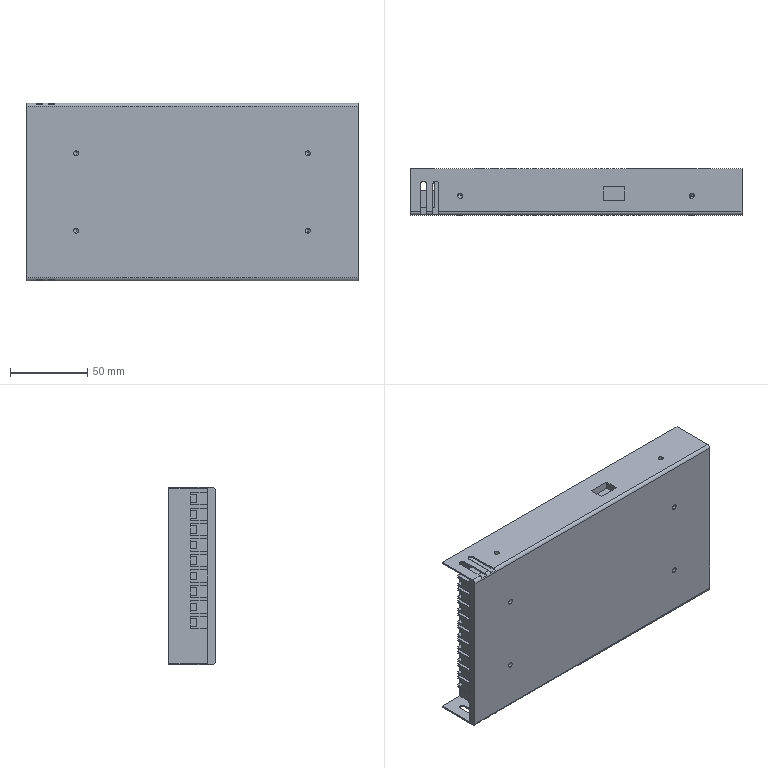Part | STEP file | Switching power supply LRS-350-48 | 11 solids | 283 faces | box 215 x 30 x 115 mm | volume 698035 mm3 | plane 163 | cylinder 104 | cone 16 | commonest cylinder face diameters 5 x60 3.3 x16 4 x6 25 x5 35 x5 45 x5